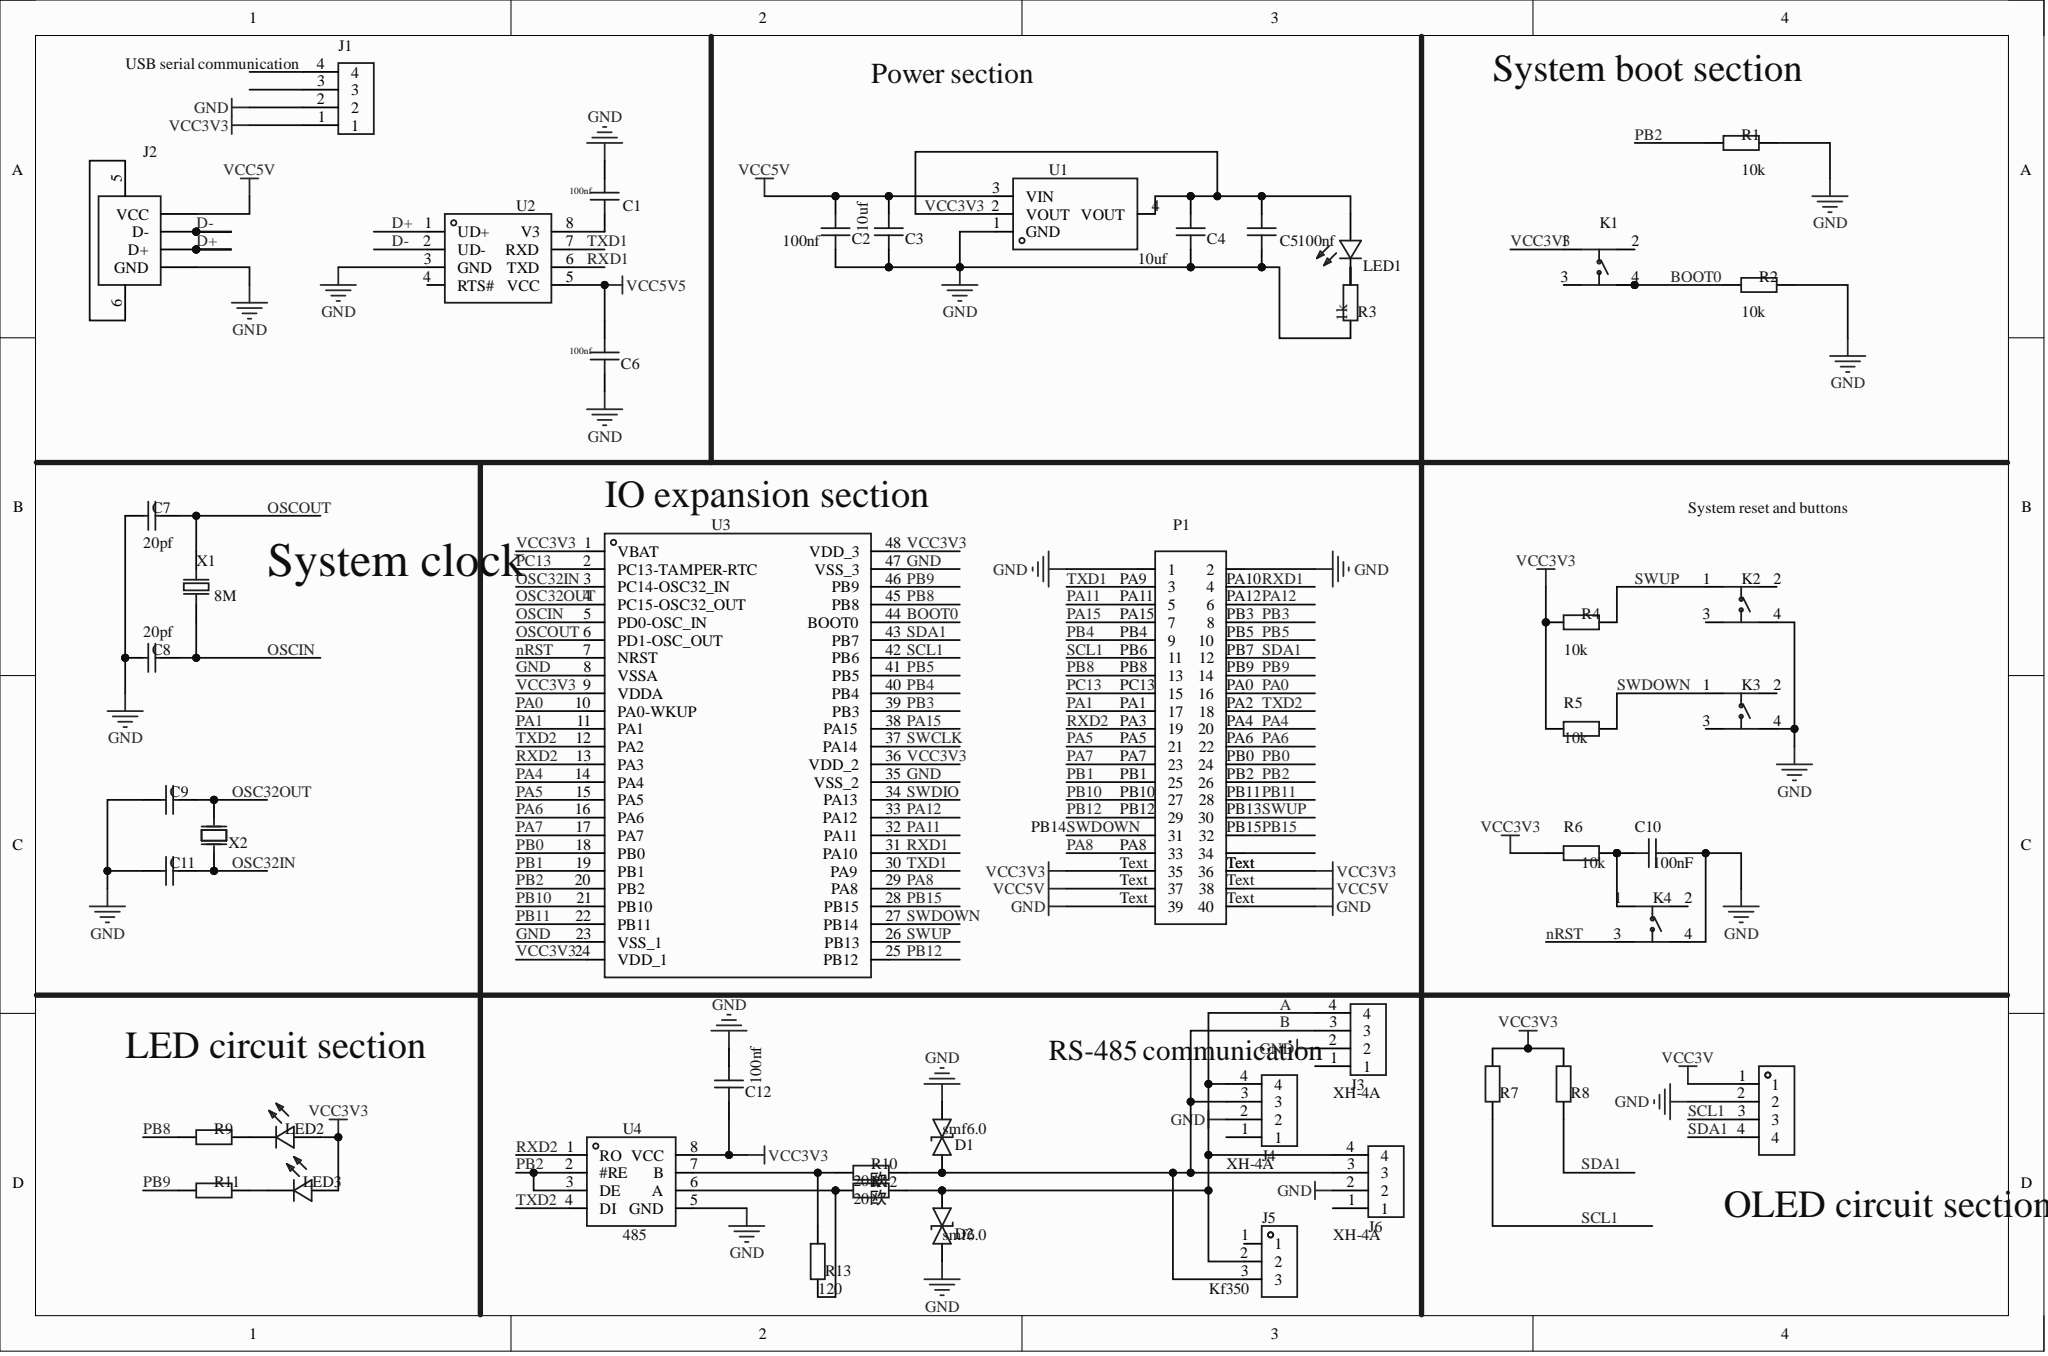Circuit board | Altium Designer | 48 parts | 53 nets
Bill of materials:
Comment,Description,Designator,Footprint,LibRef,Quantity
"CC0603KRX7R9BB104","","C1, C3, C5, C6, C12","C0603 - duplicate","CC0603KRX7R9BB104","5"
"CL21A106KAYNNNE","","C2, C4, C10","C0805","CL21A106KAYNNNE","3"
"CL10C200JB8NNNC","","C7, C8, C9, C11","C0603c20pf","CL10C200JB8NNNC","4"
"SMF6.0CA_C2990473","","D1, D2","瞬态二极管","SMF6.0CA_C2990473","2"
"PM254V-11-04-H85","","H1","排母4p","PM254V-11-04-H85","1"
"XH-4A","","J1, J3, J4, J6","XH-4A","XH-4A_1","4"
"USB-B-Female-90","","J2","USB-B_TH_USB-B-FEMALE-90","USB-B-Female-90","1"
"KF350-3.5-3P","","J5","KF350-3.5-3P","KF350-3.5-3P_1","1"
"KH-6X6X5H-STM","","K1","按键","KH-6X6X5H-STM","1"
"KH-6X6X5H-STM","","K2, K3, K4","复位按键","KH-6X6X5H-STM_1","3"
"FC-D1608HGK-572C","","LED1, LED2, LED3","LED0603-RD","FC-D1608HGK-572C","3"
"Header-Male-2.54_2x20","","P1","HDR-TH_40P-P2.54-V-M-R2-C20-S2.54","Header-Male-2.54_2x20","1"
"0603WAF1002T5E","","R1, R2, R4, R5, R6","电阻R0603","0603WAF1002T5E","5"
"0603WAF1001T5E","","R3","C0603 - duplicate","0603WAF1001T5E","1"
"0603WAF4701T5E","","R7, R8","R06034.7k","0603WAF4701T5E","2"
"0603WAF1001T5E","","R9, R11","R06031k","0603WAF1001T5E_1","2"
"0805W8F200JT5E","","R10, R12","R0805","0805W8F200JT5E","2"
"0603WAF1200T5E","","R13","R0603 - duplicate","0603WAF1200T5E","1"
"AMS1117-3.3","","U1","SOT-223-3_L6.5-W3.4-P2.30-LS7.0-BR","AMS1117-3.3","1"
"CH340N_C2977777","","U2","SOP-8_L4.9-W3.9-P1.27-LS6.0-BL","CH340N_C2977777","1"
"STM32F103C8T6","","U3","LQFP-48_L7.0-W7.0-P0.50-LS9.0-BL","STM32F103C8T6","1"
"SP3485EEN","","U4","485SOP-8_L5.0-W4.0-P1.27-LS6.0-BL","SP3485EEN","1"
"Q13FC1350000400","","X1","CRYSTAL-SMD_L5.0-W3.2","Q13FC1350000400","1"
"X50328MSB2GI","","X2","FC-135R_L3.2-W1.5","X50328MSB2GI","1"
Netlist (Protel format):
[
C1
C0603 - duplicate
CC0603KRX7R9BB104



]
[
C2
C0805
CL21A106KAYNNNE



]
[
C3
C0603 - duplicate
CC0603KRX7R9BB104



]
[
C4
C0805
CL21A106KAYNNNE



]
[
C5
C0603 - duplicate
CC0603KRX7R9BB104



]
[
C6
C0603 - duplicate
CC0603KRX7R9BB104



]
[
C7
C0603c20pf
CL10C200JB8NNNC



]
[
C8
C0603c20pf
CL10C200JB8NNNC



]
[
C9
C0603c20pf
CL10C200JB8NNNC



]
[
C10
C0805
CL21A106KAYNNNE



]
[
C11
C0603c20pf
CL10C200JB8NNNC



]
[
C12
C0603 - duplicate
CC0603KRX7R9BB104



]
[
D1
瞬态二极管
SMF6.0CA_C2990473



]
[
D2
瞬态二极管
SMF6.0CA_C2990473



]
[
H1
排母4p
PM254V-11-04-H85



]
[
J1
XH-4A
XH-4A



]
[
J2
USB-B_TH_USB-B-FEMALE-90
USB-B-Female-90



]
[
J3
XH-4A
XH-4A



]
[
J4
XH-4A
XH-4A



]
[
J5
KF350-3.5-3P
KF350-3.5-3P



]
[
J6
XH-4A
XH-4A



]
[
K1
按键
KH-6X6X5H-STM



]
[
K2
复位按键
KH-6X6X5H-STM



]
[
K3
复位按键
KH-6X6X5H-STM



]
[
K4
复位按键
KH-6X6X5H-STM



]
[
LED1
LED0603-RD
FC-D1608HGK-572C



]
[
LED2
LED0603-RD
FC-D1608HGK-572C



]
[
LED3
LED0603-RD
FC-D1608HGK-572C



]
[
P1
HDR-TH_40P-P2.54-V-M-R2-C20-S2.54
Header-Male-2.54_2x20



]
[
R1
电阻R0603
0603WAF1002T5E



]
[
R2
电阻R0603
0603WAF1002T5E



]
[
R3
C0603 - duplicate
0603WAF1001T5E



]
[
R4
电阻R0603
0603WAF1002T5E



]
[
R5
电阻R0603
0603WAF1002T5E



]
[
R6
电阻R0603
0603WAF1002T5E



]
[
R7
R06034.7k
0603WAF4701T5E



]
[
R8
R06034.7k
0603WAF4701T5E



]
[
R9
R06031k
0603WAF1001T5E



]
[
R10
R0805
0805W8F200JT5E



]
[
R11
R06031k
0603WAF1001T5E



]
[
R12
R0805
0805W8F200JT5E



]
[
R13
R0603 - duplicate
0603WAF1200T5E



]
[
U1
SOT-223-3_L6.5-W3.4-P2.30-LS7.0-BR
AMS1117-3.3



]
[
U2
SOP-8_L4.9-W3.9-P1.27-LS6.0-BL
CH340N_C2977777



]
[
U3
LQFP-48_L7.0-W7.0-P0.50-LS9.0-BL
STM32F103C8T6



]
[
U4
485SOP-8_L5.0-W4.0-P1.27-LS6.0-BL
SP3485EEN



]
[
X1
CRYSTAL-SMD_L5.0-W3.2
Q13FC1350000400



]
[
X2
FC-135R_L3.2-W1.5
X50328MSB2GI



]
(
VCC5V5
C6-2
U2-5
)
(
VCC5V
C2-2
C3-1
J2-1
P1-37
P1-38
U1-3
)
(
VCC3V3
C4-2
C5-2
C12-1
J1-1
K1-1
LED1-2
LED2-2
LED3-2
P1-35
P1-36
R4-1
R5-1
R6-1
R7-2
R8-2
U1-2
U1-4
U3-1
U3-9
U3-24
U3-36
U3-48
U4-8
)
(
TXD2
P1-18
U3-12
U4-4
)
(
TXD1
P1-3
U2-7
U3-30
)
(
SWUP
K2-1
P1-30
R4-2
U3-26
)
(
SWDOWN
K3-1
P1-31
R5-2
U3-27
)
(
SDA1
H1-4
P1-12
R8-1
U3-43
)
(
SCL1
H1-3
P1-11
R7-1
U3-42
)
(
RXD2
P1-19
U3-13
U4-1
)
(
RXD1
P1-4
U2-6
U3-31
)
(
PC13
P1-15
U3-2
)
(
PB15
P1-32
U3-28
)
(
PB12
P1-29
U3-25
)
(
PB11
P1-28
U3-22
)
(
PB10
P1-27
U3-21
)
(
PB9
P1-14
R11-1
U3-46
)
(
PB8
P1-13
R9-1
U3-45
)
(
PB5
P1-10
U3-41
)
(
PB4
P1-9
U3-40
)
(
PB3
P1-8
U3-39
)
(
PB2
P1-26
R1-1
U3-20
U4-2
U4-3
)
(
PB1
P1-25
U3-19
)
(
PB0
P1-24
U3-18
)
(
PA15
P1-7
U3-38
)
(
PA12
P1-6
U3-33
)
(
PA11
P1-5
U3-32
)
(
PA8
P1-33
U3-29
)
(
PA7
P1-23
U3-17
)
(
PA6
P1-22
U3-16
)
(
PA5
P1-21
U3-15
)
(
PA4
P1-20
U3-14
)
(
PA1
P1-17
U3-11
)
(
PA0
P1-16
U3-10
)
(
OSCOUT
C7-2
U3-6
X1-1
)
(
OSCIN
C8-2
U3-5
X1-2
)
(
OSC32OUT
C9-2
U3-4
X2-1
)
(
OSC32IN
C11-2
U3-3
X2-2
)
(
nRST
K4-3
U3-7
)
(
NetR12_1
R12-1
R13-1
U4-6
)
(
NetR10_1
R10-1
R13-2
U4-7
)
(
NetLED3_1
LED3-1
R11-2
)
(
NetLED2_1
LED2-1
R9-2
)
(
NetLED1_1
LED1-1
R3-2
)
(
NetJ2_5
J2-5
J2-6
)
(
NetC10_2
C10-2
K4-1
R6-2
)
(
NetC1_1
C1-1
U2-8
)
(
GND
C1-2
C2-1
C3-2
C4-1
C5-1
C6-1
C7-1
C8-1
C9-1
C10-1
C11-1
C12-2
D1-2
D2-1
H1-2
J1-2
J2-4
J3-2
J4-2
J6-2
K2-4
K3-4
K4-4
P1-1
P1-2
P1-39
P1-40
R1-2
R2-2
R3-1
U1-1
U2-3
U3-8
U3-23
U3-35
U3-47
U4-5
)
(
D-
J2-2
U2-2
)
(
D+
J2-3
U2-1
)
(
BOOT0
K1-4
R2-1
U3-44
)
(
B
D1-1
J3-3
J4-3
J5-3
J6-3
R10-2
)
(
A
D2-2
J3-4
J4-4
J5-2
J6-4
R12-2
)